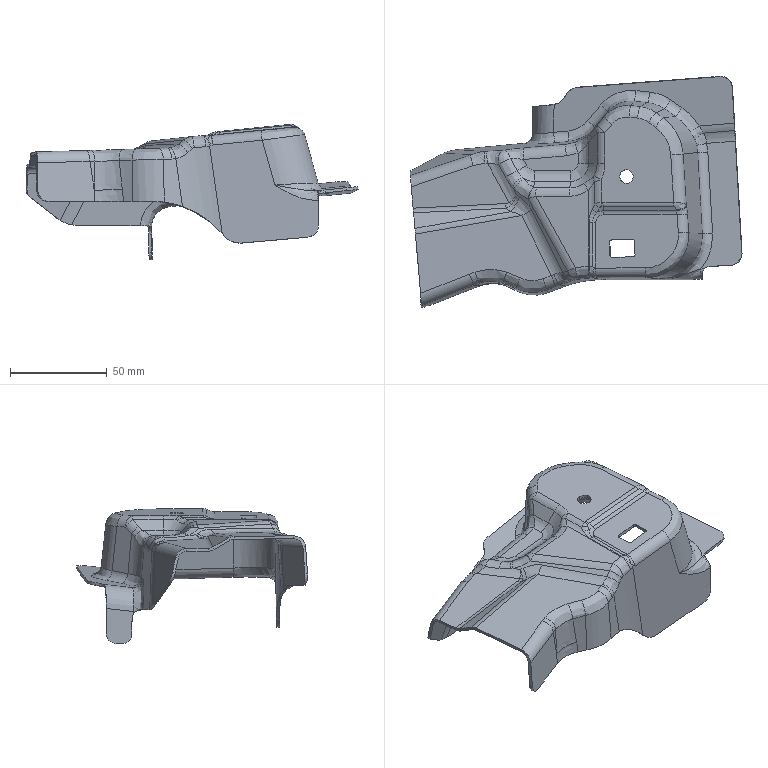Part | 1 solid | 335 faces | box 171.16 x 119.236 x 69.7 mm | volume 38591 mm3 | spline 194 | cylinder 96 | plane 38 | sphere 4 | other 3 | commonest cylinder face diameters 10 x15 9 x12 12 x12 13 x11 7 x8 2 x4